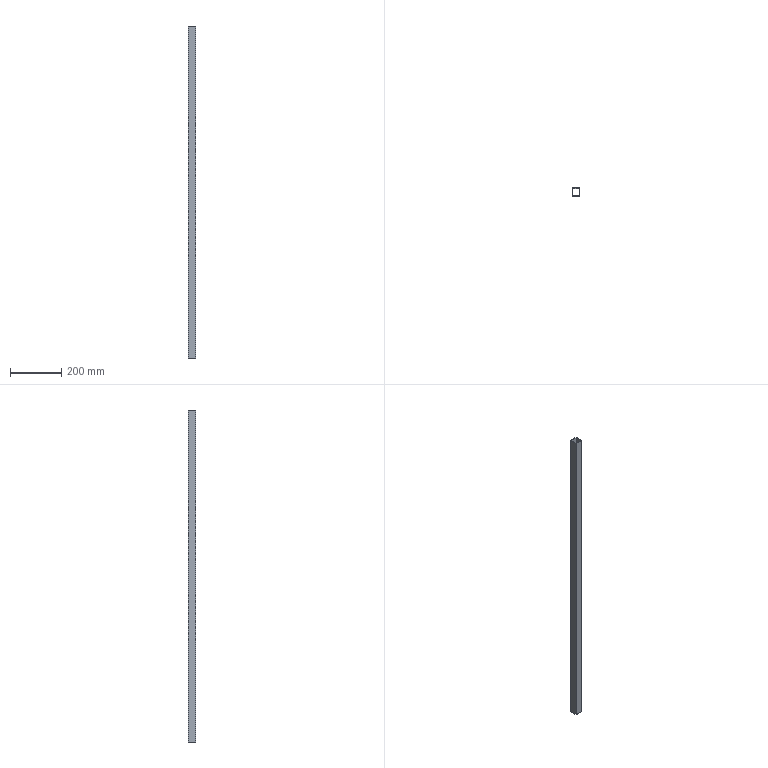Part | SolidWorks | features Extrusion 1 | 1 solid | 10 faces | box 30 x 30 x 1300 mm | volume 291200 mm3 | plane 10
STEP:
#1=CARTESIAN_POINT('',(-15.,15.,650.));
#2=VERTEX_POINT('',#1);
#3=CARTESIAN_POINT('',(-15.,-15.,650.));
#4=VERTEX_POINT('',#3);
#5=CARTESIAN_POINT('',(-15.,-15.,650.));
#6=DIRECTION('',(0.,-1.,0.));
#7=VECTOR('',#6,1000.);
#8=LINE('',#5,#7);
#9=EDGE_CURVE('',#2,#4,#8,.T.);
#10=ORIENTED_EDGE('',*,*,#9,.T.);
#11=CARTESIAN_POINT('',(15.,-15.,650.));
#12=VERTEX_POINT('',#11);
#13=CARTESIAN_POINT('',(15.,-15.,650.));
#14=DIRECTION('',(1.,0.,0.));
#15=VECTOR('',#14,1000.);
#16=LINE('',#13,#15);
#17=EDGE_CURVE('',#4,#12,#16,.T.);
#18=ORIENTED_EDGE('',*,*,#17,.T.);
#19=CARTESIAN_POINT('',(15.,15.,650.));
#20=VERTEX_POINT('',#19);
#21=CARTESIAN_POINT('',(15.,-15.,650.));
#22=DIRECTION('',(0.,1.,0.));
#23=VECTOR('',#22,1000.);
#24=LINE('',#21,#23);
#25=EDGE_CURVE('',#12,#20,#24,.T.);
#26=ORIENTED_EDGE('',*,*,#25,.T.);
#27=CARTESIAN_POINT('',(15.,15.,650.));
#28=DIRECTION('',(-1.,0.,0.));
#29=VECTOR('',#28,1000.);
#30=LINE('',#27,#29);
#31=EDGE_CURVE('',#20,#2,#30,.T.);
#32=ORIENTED_EDGE('',*,*,#31,.T.);
#33=EDGE_LOOP('',(#10,#18,#26,#32));
#34=FACE_OUTER_BOUND('',#33,.T.);
#35=CARTESIAN_POINT('',(13.,-13.,650.));
#36=VERTEX_POINT('',#35);
#37=CARTESIAN_POINT('',(13.,13.,650.));
#38=VERTEX_POINT('',#37);
#39=CARTESIAN_POINT('',(13.,-13.,650.));
#40=DIRECTION('',(0.,1.,0.));
#41=VECTOR('',#40,1000.);
#42=LINE('',#39,#41);
#43=EDGE_CURVE('',#36,#38,#42,.T.);
#44=ORIENTED_EDGE('',*,*,#43,.F.);
#45=CARTESIAN_POINT('',(-13.,-13.,650.));
#46=VERTEX_POINT('',#45);
#47=CARTESIAN_POINT('',(13.,-13.,650.));
#48=DIRECTION('',(1.,0.,0.));
#49=VECTOR('',#48,1000.);
#50=LINE('',#47,#49);
#51=EDGE_CURVE('',#46,#36,#50,.T.);
#52=ORIENTED_EDGE('',*,*,#51,.F.);
#53=CARTESIAN_POINT('',(-13.,13.,650.));
#54=VERTEX_POINT('',#53);
#55=CARTESIAN_POINT('',(-13.,-13.,650.));
#56=DIRECTION('',(0.,-1.,0.));
#57=VECTOR('',#56,1000.);
#58=LINE('',#55,#57);
#59=EDGE_CURVE('',#54,#46,#58,.T.);
#60=ORIENTED_EDGE('',*,*,#59,.F.);
#61=CARTESIAN_POINT('',(13.,13.,650.));
#62=DIRECTION('',(-1.,0.,0.));
#63=VECTOR('',#62,1000.);
#64=LINE('',#61,#63);
#65=EDGE_CURVE('',#38,#54,#64,.T.);
#66=ORIENTED_EDGE('',*,*,#65,.F.);
#67=EDGE_LOOP('',(#44,#52,#60,#66));
#68=FACE_BOUND('',#67,.T.);
#69=CARTESIAN_POINT('',(0.,0.,650.));
#70=DIRECTION('',(0.,0.,1.));
#71=DIRECTION('',(1.,0.,0.));
#72=AXIS2_PLACEMENT_3D('',#69,#70,#71);
#73=PLANE('',#72);
#74=ADVANCED_FACE('',(#34,#68),#73,.T.);
#75=CARTESIAN_POINT('',(-15.,15.,-650.));
#76=VERTEX_POINT('',#75);
#77=CARTESIAN_POINT('',(-15.,-15.,-650.));
#78=VERTEX_POINT('',#77);
#79=CARTESIAN_POINT('',(-15.,-15.,-650.));
#80=DIRECTION('',(0.,-1.,0.));
#81=VECTOR('',#80,1000.);
#82=LINE('',#79,#81);
#83=EDGE_CURVE('',#76,#78,#82,.T.);
#84=ORIENTED_EDGE('',*,*,#83,.F.);
#85=CARTESIAN_POINT('',(15.,15.,-650.));
#86=VERTEX_POINT('',#85);
#87=CARTESIAN_POINT('',(15.,15.,-650.));
#88=DIRECTION('',(-1.,0.,0.));
#89=VECTOR('',#88,1000.);
#90=LINE('',#87,#89);
#91=EDGE_CURVE('',#86,#76,#90,.T.);
#92=ORIENTED_EDGE('',*,*,#91,.F.);
#93=CARTESIAN_POINT('',(15.,-15.,-650.));
#94=VERTEX_POINT('',#93);
#95=CARTESIAN_POINT('',(15.,-15.,-650.));
#96=DIRECTION('',(0.,1.,0.));
#97=VECTOR('',#96,1000.);
#98=LINE('',#95,#97);
#99=EDGE_CURVE('',#94,#86,#98,.T.);
#100=ORIENTED_EDGE('',*,*,#99,.F.);
#101=CARTESIAN_POINT('',(15.,-15.,-650.));
#102=DIRECTION('',(1.,0.,0.));
#103=VECTOR('',#102,1000.);
#104=LINE('',#101,#103);
#105=EDGE_CURVE('',#78,#94,#104,.T.);
#106=ORIENTED_EDGE('',*,*,#105,.F.);
#107=EDGE_LOOP('',(#84,#92,#100,#106));
#108=FACE_OUTER_BOUND('',#107,.T.);
#109=CARTESIAN_POINT('',(-13.,-13.,-650.));
#110=VERTEX_POINT('',#109);
#111=CARTESIAN_POINT('',(13.,-13.,-650.));
#112=VERTEX_POINT('',#111);
#113=CARTESIAN_POINT('',(13.,-13.,-650.));
#114=DIRECTION('',(1.,0.,0.));
#115=VECTOR('',#114,1000.);
#116=LINE('',#113,#115);
#117=EDGE_CURVE('',#110,#112,#116,.T.);
#118=ORIENTED_EDGE('',*,*,#117,.T.);
#119=CARTESIAN_POINT('',(13.,13.,-650.));
#120=VERTEX_POINT('',#119);
#121=CARTESIAN_POINT('',(13.,-13.,-650.));
#122=DIRECTION('',(0.,1.,0.));
#123=VECTOR('',#122,1000.);
#124=LINE('',#121,#123);
#125=EDGE_CURVE('',#112,#120,#124,.T.);
#126=ORIENTED_EDGE('',*,*,#125,.T.);
#127=CARTESIAN_POINT('',(-13.,13.,-650.));
#128=VERTEX_POINT('',#127);
#129=CARTESIAN_POINT('',(13.,13.,-650.));
#130=DIRECTION('',(-1.,0.,0.));
#131=VECTOR('',#130,1000.);
#132=LINE('',#129,#131);
#133=EDGE_CURVE('',#120,#128,#132,.T.);
#134=ORIENTED_EDGE('',*,*,#133,.T.);
#135=CARTESIAN_POINT('',(-13.,-13.,-650.));
#136=DIRECTION('',(0.,-1.,0.));
#137=VECTOR('',#136,1000.);
#138=LINE('',#135,#137);
#139=EDGE_CURVE('',#128,#110,#138,.T.);
#140=ORIENTED_EDGE('',*,*,#139,.T.);
#141=EDGE_LOOP('',(#118,#126,#134,#140));
#142=FACE_BOUND('',#141,.T.);
#143=CARTESIAN_POINT('',(0.,0.,-650.));
#144=DIRECTION('',(0.,0.,1.));
#145=DIRECTION('',(1.,0.,0.));
#146=AXIS2_PLACEMENT_3D('',#143,#144,#145);
#147=PLANE('',#146);
#148=ADVANCED_FACE('',(#108,#142),#147,.F.);
#149=ORIENTED_EDGE('',*,*,#83,.T.);
#150=CARTESIAN_POINT('',(-15.,-15.,650.));
#151=DIRECTION('',(0.,0.,-1.));
#152=VECTOR('',#151,1000.);
#153=LINE('',#150,#152);
#154=EDGE_CURVE('',#4,#78,#153,.T.);
#155=ORIENTED_EDGE('',*,*,#154,.F.);
#156=ORIENTED_EDGE('',*,*,#9,.F.);
#157=CARTESIAN_POINT('',(-15.,15.,650.));
#158=DIRECTION('',(0.,0.,-1.));
#159=VECTOR('',#158,1000.);
#160=LINE('',#157,#159);
#161=EDGE_CURVE('',#2,#76,#160,.T.);
#162=ORIENTED_EDGE('',*,*,#161,.T.);
#163=EDGE_LOOP('',(#149,#155,#156,#162));
#164=FACE_OUTER_BOUND('',#163,.T.);
#165=CARTESIAN_POINT('',(-15.,-15.,650.));
#166=DIRECTION('',(1.,0.,0.));
#167=DIRECTION('',(0.,1.,0.));
#168=AXIS2_PLACEMENT_3D('',#165,#166,#167);
#169=PLANE('',#168);
#170=ADVANCED_FACE('',(#164),#169,.F.);
#171=ORIENTED_EDGE('',*,*,#105,.T.);
#172=CARTESIAN_POINT('',(15.,-15.,650.));
#173=DIRECTION('',(0.,0.,-1.));
#174=VECTOR('',#173,1000.);
#175=LINE('',#172,#174);
#176=EDGE_CURVE('',#12,#94,#175,.T.);
#177=ORIENTED_EDGE('',*,*,#176,.F.);
#178=ORIENTED_EDGE('',*,*,#17,.F.);
#179=ORIENTED_EDGE('',*,*,#154,.T.);
#180=EDGE_LOOP('',(#171,#177,#178,#179));
#181=FACE_OUTER_BOUND('',#180,.T.);
#182=CARTESIAN_POINT('',(15.,-15.,650.));
#183=DIRECTION('',(0.,1.,0.));
#184=DIRECTION('',(-1.,0.,0.));
#185=AXIS2_PLACEMENT_3D('',#182,#183,#184);
#186=PLANE('',#185);
#187=ADVANCED_FACE('',(#181),#186,.F.);
#188=ORIENTED_EDGE('',*,*,#99,.T.);
#189=CARTESIAN_POINT('',(15.,15.,650.));
#190=DIRECTION('',(0.,0.,-1.));
#191=VECTOR('',#190,1000.);
#192=LINE('',#189,#191);
#193=EDGE_CURVE('',#20,#86,#192,.T.);
#194=ORIENTED_EDGE('',*,*,#193,.F.);
#195=ORIENTED_EDGE('',*,*,#25,.F.);
#196=ORIENTED_EDGE('',*,*,#176,.T.);
#197=EDGE_LOOP('',(#188,#194,#195,#196));
#198=FACE_OUTER_BOUND('',#197,.T.);
#199=CARTESIAN_POINT('',(15.,-15.,650.));
#200=DIRECTION('',(-1.,0.,0.));
#201=DIRECTION('',(0.,0.,1.));
#202=AXIS2_PLACEMENT_3D('',#199,#200,#201);
#203=PLANE('',#202);
#204=ADVANCED_FACE('',(#198),#203,.F.);
#205=ORIENTED_EDGE('',*,*,#91,.T.);
#206=ORIENTED_EDGE('',*,*,#161,.F.);
#207=ORIENTED_EDGE('',*,*,#31,.F.);
#208=ORIENTED_EDGE('',*,*,#193,.T.);
#209=EDGE_LOOP('',(#205,#206,#207,#208));
#210=FACE_OUTER_BOUND('',#209,.T.);
#211=CARTESIAN_POINT('',(15.,15.,650.));
#212=DIRECTION('',(0.,-1.,0.));
#213=DIRECTION('',(0.,0.,-1.));
#214=AXIS2_PLACEMENT_3D('',#211,#212,#213);
#215=PLANE('',#214);
#216=ADVANCED_FACE('',(#210),#215,.F.);
#217=ORIENTED_EDGE('',*,*,#117,.F.);
#218=CARTESIAN_POINT('',(-13.,-13.,650.));
#219=DIRECTION('',(0.,0.,-1.));
#220=VECTOR('',#219,1000.);
#221=LINE('',#218,#220);
#222=EDGE_CURVE('',#46,#110,#221,.T.);
#223=ORIENTED_EDGE('',*,*,#222,.F.);
#224=ORIENTED_EDGE('',*,*,#51,.T.);
#225=CARTESIAN_POINT('',(13.,-13.,650.));
#226=DIRECTION('',(0.,0.,-1.));
#227=VECTOR('',#226,1000.);
#228=LINE('',#225,#227);
#229=EDGE_CURVE('',#36,#112,#228,.T.);
#230=ORIENTED_EDGE('',*,*,#229,.T.);
#231=EDGE_LOOP('',(#217,#223,#224,#230));
#232=FACE_OUTER_BOUND('',#231,.T.);
#233=CARTESIAN_POINT('',(13.,-13.,650.));
#234=DIRECTION('',(0.,1.,0.));
#235=DIRECTION('',(0.,0.,1.));
#236=AXIS2_PLACEMENT_3D('',#233,#234,#235);
#237=PLANE('',#236);
#238=ADVANCED_FACE('',(#232),#237,.T.);
#239=ORIENTED_EDGE('',*,*,#125,.F.);
#240=ORIENTED_EDGE('',*,*,#229,.F.);
#241=ORIENTED_EDGE('',*,*,#43,.T.);
#242=CARTESIAN_POINT('',(13.,13.,650.));
#243=DIRECTION('',(0.,0.,-1.));
#244=VECTOR('',#243,1000.);
#245=LINE('',#242,#244);
#246=EDGE_CURVE('',#38,#120,#245,.T.);
#247=ORIENTED_EDGE('',*,*,#246,.T.);
#248=EDGE_LOOP('',(#239,#240,#241,#247));
#249=FACE_OUTER_BOUND('',#248,.T.);
#250=CARTESIAN_POINT('',(13.,-13.,650.));
#251=DIRECTION('',(-1.,0.,0.));
#252=DIRECTION('',(0.,0.,1.));
#253=AXIS2_PLACEMENT_3D('',#250,#251,#252);
#254=PLANE('',#253);
#255=ADVANCED_FACE('',(#249),#254,.T.);
#256=ORIENTED_EDGE('',*,*,#133,.F.);
#257=ORIENTED_EDGE('',*,*,#246,.F.);
#258=ORIENTED_EDGE('',*,*,#65,.T.);
#259=CARTESIAN_POINT('',(-13.,13.,650.));
#260=DIRECTION('',(0.,0.,-1.));
#261=VECTOR('',#260,1000.);
#262=LINE('',#259,#261);
#263=EDGE_CURVE('',#54,#128,#262,.T.);
#264=ORIENTED_EDGE('',*,*,#263,.T.);
#265=EDGE_LOOP('',(#256,#257,#258,#264));
#266=FACE_OUTER_BOUND('',#265,.T.);
#267=CARTESIAN_POINT('',(13.,13.,650.));
#268=DIRECTION('',(0.,-1.,0.));
#269=DIRECTION('',(0.,0.,-1.));
#270=AXIS2_PLACEMENT_3D('',#267,#268,#269);
#271=PLANE('',#270);
#272=ADVANCED_FACE('',(#266),#271,.T.);
#273=ORIENTED_EDGE('',*,*,#139,.F.);
#274=ORIENTED_EDGE('',*,*,#263,.F.);
#275=ORIENTED_EDGE('',*,*,#59,.T.);
#276=ORIENTED_EDGE('',*,*,#222,.T.);
#277=EDGE_LOOP('',(#273,#274,#275,#276));
#278=FACE_OUTER_BOUND('',#277,.T.);
#279=CARTESIAN_POINT('',(-13.,-13.,650.));
#280=DIRECTION('',(1.,0.,0.));
#281=DIRECTION('',(0.,0.,-1.));
#282=AXIS2_PLACEMENT_3D('',#279,#280,#281);
#283=PLANE('',#282);
#284=ADVANCED_FACE('',(#278),#283,.T.);
#285=CLOSED_SHELL('',(#74,#148,#170,#187,#204,#216,#238,#255,#272,#284));
#286=MANIFOLD_SOLID_BREP('',#285);
#287=CARTESIAN_POINT('',(0.,0.,0.));
#288=DIRECTION('',(0.,0.,1.));
#289=DIRECTION('',(1.,0.,0.));
#290=AXIS2_PLACEMENT_3D('',#287,#288,#289);
#291=(LENGTH_UNIT()NAMED_UNIT(*)SI_UNIT(.MILLI.,.METRE.));
#292=UNCERTAINTY_MEASURE_WITH_UNIT(LENGTH_MEASURE(0.00001),#291,'','');
#293=(NAMED_UNIT(*)PLANE_ANGLE_UNIT()SI_UNIT($,.RADIAN.));
#294=(NAMED_UNIT(*)SI_UNIT($,.STERADIAN.)SOLID_ANGLE_UNIT());
#295=(GEOMETRIC_REPRESENTATION_CONTEXT(3)GLOBAL_UNCERTAINTY_ASSIGNED_CONTEXT((#292))GLOBAL_UNIT_ASSIGNED_CONTEXT((#291,#293,#294))REPRESENTATION_CONTEXT('',''));
#296=ADVANCED_BREP_SHAPE_REPRESENTATION('',(#286,#290),#295);